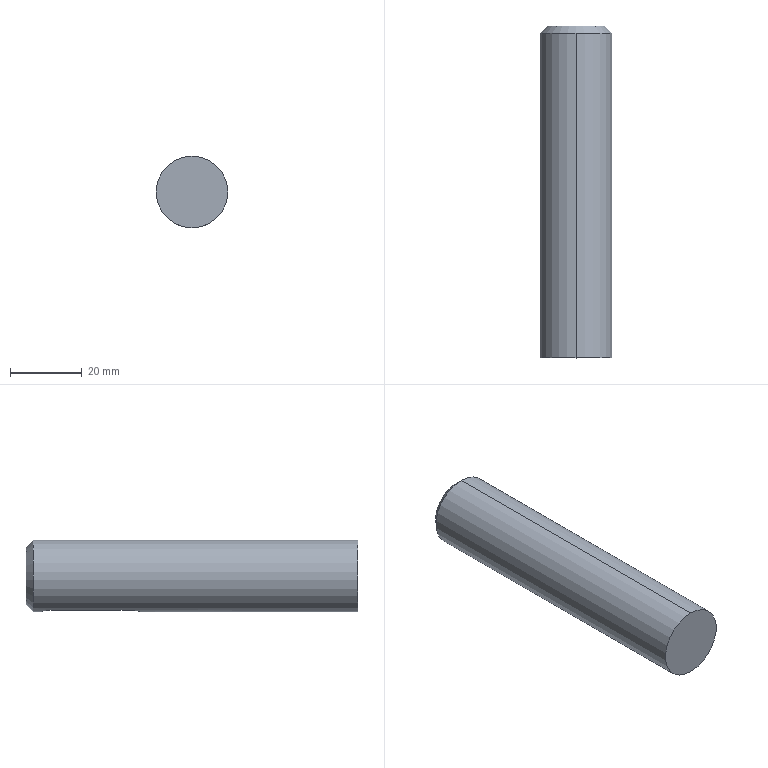Part | SolidWorks | features Chamfer 1, Extrusion 1, ICE 1 | 1 solid | 11 faces | box 20 x 92.5 x 20 mm | volume 28405 mm3 | plane 5 | cylinder 4 | cone 2 | commonest cylinder face diameters 6 x2 20 x2
STEP:
#1=CARTESIAN_POINT('',(0.,92.5,8.));
#2=VERTEX_POINT('',#1);
#3=CARTESIAN_POINT('',(0.,92.5,-8.));
#4=VERTEX_POINT('',#3);
#5=CARTESIAN_POINT('',(0.,92.5,0.));
#6=DIRECTION('',(0.,1.,0.));
#7=DIRECTION('',(0.,0.,1.));
#8=AXIS2_PLACEMENT_3D('',#5,#6,#7);
#9=CIRCLE('',#8,8.);
#10=EDGE_CURVE('',#2,#4,#9,.T.);
#11=ORIENTED_EDGE('',*,*,#10,.F.);
#12=CARTESIAN_POINT('',(0.,90.5,10.));
#13=VERTEX_POINT('',#12);
#14=CARTESIAN_POINT('',(0.,92.5,8.));
#15=DIRECTION('',(0.,-0.7071,0.7071));
#16=VECTOR('',#15,1000.);
#17=LINE('',#14,#16);
#18=EDGE_CURVE('',#2,#13,#17,.T.);
#19=ORIENTED_EDGE('',*,*,#18,.T.);
#20=CARTESIAN_POINT('',(0.,90.5,-10.));
#21=VERTEX_POINT('',#20);
#22=CARTESIAN_POINT('',(0.,90.5,0.));
#23=DIRECTION('',(0.,-1.,0.));
#24=DIRECTION('',(0.,0.,1.));
#25=AXIS2_PLACEMENT_3D('',#22,#23,#24);
#26=CIRCLE('',#25,10.);
#27=EDGE_CURVE('',#21,#13,#26,.T.);
#28=ORIENTED_EDGE('',*,*,#27,.F.);
#29=CARTESIAN_POINT('',(0.,92.5,-8.));
#30=DIRECTION('',(0.,-0.7071,-0.7071));
#31=VECTOR('',#30,1000.);
#32=LINE('',#29,#31);
#33=EDGE_CURVE('',#4,#21,#32,.T.);
#34=ORIENTED_EDGE('',*,*,#33,.F.);
#35=EDGE_LOOP('',(#11,#19,#28,#34));
#36=FACE_OUTER_BOUND('',#35,.T.);
#37=CARTESIAN_POINT('',(0.,92.5,0.));
#38=DIRECTION('',(0.,-1.,0.));
#39=DIRECTION('',(0.,0.,-1.));
#40=AXIS2_PLACEMENT_3D('',#37,#38,#39);
#41=CONICAL_SURFACE('',#40,8.,0.7854);
#42=ADVANCED_FACE('',(#36),#41,.T.);
#43=ORIENTED_EDGE('',*,*,#27,.T.);
#44=CARTESIAN_POINT('',(0.,0.,10.));
#45=VERTEX_POINT('',#44);
#46=CARTESIAN_POINT('',(0.,92.5,10.));
#47=DIRECTION('',(0.,-1.,0.));
#48=VECTOR('',#47,1000.);
#49=LINE('',#46,#48);
#50=EDGE_CURVE('',#13,#45,#49,.T.);
#51=ORIENTED_EDGE('',*,*,#50,.T.);
#52=CARTESIAN_POINT('',(0.,0.,-10.));
#53=VERTEX_POINT('',#52);
#54=CARTESIAN_POINT('',(0.,0.,0.));
#55=DIRECTION('',(0.,1.,0.));
#56=DIRECTION('',(0.,0.,1.));
#57=AXIS2_PLACEMENT_3D('',#54,#55,#56);
#58=CIRCLE('',#57,10.);
#59=EDGE_CURVE('',#45,#53,#58,.T.);
#60=ORIENTED_EDGE('',*,*,#59,.T.);
#61=CARTESIAN_POINT('',(0.,60.5,-10.));
#62=VERTEX_POINT('',#61);
#63=CARTESIAN_POINT('',(0.,92.5,-10.));
#64=DIRECTION('',(0.,-1.,0.));
#65=VECTOR('',#64,1000.);
#66=LINE('',#63,#65);
#67=EDGE_CURVE('',#62,#53,#66,.T.);
#68=ORIENTED_EDGE('',*,*,#67,.F.);
#69=CARTESIAN_POINT('',(3.,63.5,-9.539));
#70=VERTEX_POINT('',#69);
#71=CARTESIAN_POINT('',(0.,60.5,-10.));
#72=CARTESIAN_POINT('',(0.1968,60.5,-10.));
#73=CARTESIAN_POINT('',(0.3967,60.52,-9.994));
#74=CARTESIAN_POINT('',(0.7821,60.597,-9.971));
#75=CARTESIAN_POINT('',(0.9695,60.654,-9.955));
#76=CARTESIAN_POINT('',(1.334,60.806,-9.912));
#77=CARTESIAN_POINT('',(1.507,60.899,-9.887));
#78=CARTESIAN_POINT('',(1.831,61.116,-9.832));
#79=CARTESIAN_POINT('',(1.983,61.241,-9.802));
#80=CARTESIAN_POINT('',(2.26,61.517,-9.742));
#81=CARTESIAN_POINT('',(2.383,61.667,-9.713));
#82=CARTESIAN_POINT('',(2.6,61.991,-9.657));
#83=CARTESIAN_POINT('',(2.694,62.167,-9.63));
#84=CARTESIAN_POINT('',(2.845,62.528,-9.587));
#85=CARTESIAN_POINT('',(2.902,62.715,-9.57));
#86=CARTESIAN_POINT('',(2.98,63.101,-9.546));
#87=CARTESIAN_POINT('',(3.,63.301,-9.539));
#88=CARTESIAN_POINT('',(3.,63.5,-9.539));
#89=B_SPLINE_CURVE_WITH_KNOTS('',3,(#71,#72,#73,#74,#75,#76,#77,#78,#79,#80,#81,#82,#83,#84,#85,#86,#87,#88),.UNSPECIFIED.,.F.,.F.,(4,2,2,2,2,2,2,2,4),(0.004718,0.005307,0.005896,0.006485,0.007074,0.007663,0.008252,0.008842,0.009431),.UNSPECIFIED.);
#90=EDGE_CURVE('',#62,#70,#89,.T.);
#91=ORIENTED_EDGE('',*,*,#90,.T.);
#92=CARTESIAN_POINT('',(3.,85.5,-9.539));
#93=VERTEX_POINT('',#92);
#94=CARTESIAN_POINT('',(3.,92.5,-9.539));
#95=DIRECTION('',(0.,1.,0.));
#96=VECTOR('',#95,1000.);
#97=LINE('',#94,#96);
#98=EDGE_CURVE('',#70,#93,#97,.T.);
#99=ORIENTED_EDGE('',*,*,#98,.T.);
#100=CARTESIAN_POINT('',(0.,88.5,-10.));
#101=VERTEX_POINT('',#100);
#102=CARTESIAN_POINT('',(3.,85.5,-9.539));
#103=CARTESIAN_POINT('',(3.,85.7,-9.539));
#104=CARTESIAN_POINT('',(2.98,85.895,-9.546));
#105=CARTESIAN_POINT('',(2.903,86.281,-9.569));
#106=CARTESIAN_POINT('',(2.845,86.472,-9.587));
#107=CARTESIAN_POINT('',(2.694,86.835,-9.631));
#108=CARTESIAN_POINT('',(2.602,87.006,-9.656));
#109=CARTESIAN_POINT('',(2.384,87.332,-9.712));
#110=CARTESIAN_POINT('',(2.258,87.485,-9.743));
#111=CARTESIAN_POINT('',(1.845,87.897,-9.832));
#112=CARTESIAN_POINT('',(1.512,88.12,-9.892));
#113=CARTESIAN_POINT('',(0.971,88.345,-9.954));
#114=CARTESIAN_POINT('',(0.7806,88.403,-9.971));
#115=CARTESIAN_POINT('',(0.3926,88.481,-9.994));
#116=CARTESIAN_POINT('',(0.197,88.5,-10.));
#117=CARTESIAN_POINT('',(0.,88.5,-10.));
#118=B_SPLINE_CURVE_WITH_KNOTS('',3,(#102,#103,#104,#105,#106,#107,#108,#109,#110,#111,#112,#113,#114,#115,#116,#117),.UNSPECIFIED.,.F.,.F.,(4,2,2,2,2,2,2,4),(0.,0.0005898,0.00118,0.001769,0.002359,0.003539,0.004128,0.004718),.UNSPECIFIED.);
#119=EDGE_CURVE('',#93,#101,#118,.T.);
#120=ORIENTED_EDGE('',*,*,#119,.T.);
#121=CARTESIAN_POINT('',(0.,92.5,-10.));
#122=DIRECTION('',(0.,-1.,0.));
#123=VECTOR('',#122,1000.);
#124=LINE('',#121,#123);
#125=EDGE_CURVE('',#21,#101,#124,.T.);
#126=ORIENTED_EDGE('',*,*,#125,.F.);
#127=EDGE_LOOP('',(#43,#51,#60,#68,#91,#99,#120,#126));
#128=FACE_OUTER_BOUND('',#127,.T.);
#129=CARTESIAN_POINT('',(0.,92.5,0.));
#130=DIRECTION('',(0.,-1.,0.));
#131=DIRECTION('',(0.,0.,-1.));
#132=AXIS2_PLACEMENT_3D('',#129,#130,#131);
#133=CYLINDRICAL_SURFACE('',#132,10.);
#134=ADVANCED_FACE('',(#128),#133,.T.);
#135=ORIENTED_EDGE('',*,*,#50,.F.);
#136=CARTESIAN_POINT('',(0.,90.5,0.));
#137=DIRECTION('',(0.,-1.,0.));
#138=DIRECTION('',(0.,0.,1.));
#139=AXIS2_PLACEMENT_3D('',#136,#137,#138);
#140=CIRCLE('',#139,10.);
#141=EDGE_CURVE('',#13,#21,#140,.T.);
#142=ORIENTED_EDGE('',*,*,#141,.T.);
#143=ORIENTED_EDGE('',*,*,#125,.T.);
#144=CARTESIAN_POINT('',(-3.,85.5,-9.539));
#145=VERTEX_POINT('',#144);
#146=CARTESIAN_POINT('',(0.,88.5,-10.));
#147=CARTESIAN_POINT('',(-0.1968,88.5,-10.));
#148=CARTESIAN_POINT('',(-0.3967,88.48,-9.994));
#149=CARTESIAN_POINT('',(-0.7821,88.403,-9.971));
#150=CARTESIAN_POINT('',(-0.9695,88.346,-9.955));
#151=CARTESIAN_POINT('',(-1.334,88.194,-9.912));
#152=CARTESIAN_POINT('',(-1.507,88.101,-9.887));
#153=CARTESIAN_POINT('',(-1.831,87.884,-9.832));
#154=CARTESIAN_POINT('',(-1.983,87.759,-9.802));
#155=CARTESIAN_POINT('',(-2.26,87.483,-9.742));
#156=CARTESIAN_POINT('',(-2.383,87.333,-9.713));
#157=CARTESIAN_POINT('',(-2.6,87.009,-9.657));
#158=CARTESIAN_POINT('',(-2.694,86.833,-9.63));
#159=CARTESIAN_POINT('',(-2.845,86.472,-9.587));
#160=CARTESIAN_POINT('',(-2.902,86.285,-9.57));
#161=CARTESIAN_POINT('',(-2.98,85.899,-9.546));
#162=CARTESIAN_POINT('',(-3.,85.699,-9.539));
#163=CARTESIAN_POINT('',(-3.,85.5,-9.539));
#164=B_SPLINE_CURVE_WITH_KNOTS('',3,(#146,#147,#148,#149,#150,#151,#152,#153,#154,#155,#156,#157,#158,#159,#160,#161,#162,#163),.UNSPECIFIED.,.F.,.F.,(4,2,2,2,2,2,2,2,4),(0.004718,0.005307,0.005896,0.006485,0.007074,0.007663,0.008252,0.008842,0.009431),.UNSPECIFIED.);
#165=EDGE_CURVE('',#101,#145,#164,.T.);
#166=ORIENTED_EDGE('',*,*,#165,.T.);
#167=CARTESIAN_POINT('',(-3.,63.5,-9.539));
#168=VERTEX_POINT('',#167);
#169=CARTESIAN_POINT('',(-3.,92.5,-9.539));
#170=DIRECTION('',(0.,-1.,0.));
#171=VECTOR('',#170,1000.);
#172=LINE('',#169,#171);
#173=EDGE_CURVE('',#145,#168,#172,.T.);
#174=ORIENTED_EDGE('',*,*,#173,.T.);
#175=CARTESIAN_POINT('',(-3.,63.5,-9.539));
#176=CARTESIAN_POINT('',(-3.,63.3,-9.539));
#177=CARTESIAN_POINT('',(-2.98,63.105,-9.546));
#178=CARTESIAN_POINT('',(-2.903,62.719,-9.569));
#179=CARTESIAN_POINT('',(-2.845,62.528,-9.587));
#180=CARTESIAN_POINT('',(-2.694,62.165,-9.631));
#181=CARTESIAN_POINT('',(-2.602,61.994,-9.656));
#182=CARTESIAN_POINT('',(-2.384,61.668,-9.712));
#183=CARTESIAN_POINT('',(-2.258,61.515,-9.743));
#184=CARTESIAN_POINT('',(-1.845,61.103,-9.832));
#185=CARTESIAN_POINT('',(-1.512,60.88,-9.892));
#186=CARTESIAN_POINT('',(-0.971,60.655,-9.954));
#187=CARTESIAN_POINT('',(-0.7806,60.597,-9.971));
#188=CARTESIAN_POINT('',(-0.3926,60.519,-9.994));
#189=CARTESIAN_POINT('',(-0.197,60.5,-10.));
#190=CARTESIAN_POINT('',(0.,60.5,-10.));
#191=B_SPLINE_CURVE_WITH_KNOTS('',3,(#175,#176,#177,#178,#179,#180,#181,#182,#183,#184,#185,#186,#187,#188,#189,#190),.UNSPECIFIED.,.F.,.F.,(4,2,2,2,2,2,2,4),(0.,0.0005898,0.00118,0.001769,0.002359,0.003539,0.004128,0.004718),.UNSPECIFIED.);
#192=EDGE_CURVE('',#168,#62,#191,.T.);
#193=ORIENTED_EDGE('',*,*,#192,.T.);
#194=ORIENTED_EDGE('',*,*,#67,.T.);
#195=CARTESIAN_POINT('',(0.,0.,0.));
#196=DIRECTION('',(0.,1.,0.));
#197=DIRECTION('',(0.,0.,1.));
#198=AXIS2_PLACEMENT_3D('',#195,#196,#197);
#199=CIRCLE('',#198,10.);
#200=EDGE_CURVE('',#53,#45,#199,.T.);
#201=ORIENTED_EDGE('',*,*,#200,.T.);
#202=EDGE_LOOP('',(#135,#142,#143,#166,#174,#193,#194,#201));
#203=FACE_OUTER_BOUND('',#202,.T.);
#204=CARTESIAN_POINT('',(0.,92.5,0.));
#205=DIRECTION('',(0.,-1.,0.));
#206=DIRECTION('',(0.,0.,-1.));
#207=AXIS2_PLACEMENT_3D('',#204,#205,#206);
#208=CYLINDRICAL_SURFACE('',#207,10.);
#209=ADVANCED_FACE('',(#203),#208,.T.);
#210=CARTESIAN_POINT('',(0.,92.5,0.));
#211=DIRECTION('',(0.,1.,0.));
#212=DIRECTION('',(0.,0.,1.));
#213=AXIS2_PLACEMENT_3D('',#210,#211,#212);
#214=CIRCLE('',#213,8.);
#215=EDGE_CURVE('',#4,#2,#214,.T.);
#216=ORIENTED_EDGE('',*,*,#215,.T.);
#217=ORIENTED_EDGE('',*,*,#10,.T.);
#218=EDGE_LOOP('',(#216,#217));
#219=FACE_OUTER_BOUND('',#218,.T.);
#220=CARTESIAN_POINT('',(0.,92.5,0.));
#221=DIRECTION('',(0.,1.,0.));
#222=DIRECTION('',(0.,0.,1.));
#223=AXIS2_PLACEMENT_3D('',#220,#221,#222);
#224=PLANE('',#223);
#225=ADVANCED_FACE('',(#219),#224,.T.);
#226=ORIENTED_EDGE('',*,*,#200,.F.);
#227=ORIENTED_EDGE('',*,*,#59,.F.);
#228=EDGE_LOOP('',(#226,#227));
#229=FACE_OUTER_BOUND('',#228,.T.);
#230=CARTESIAN_POINT('',(0.,0.,0.));
#231=DIRECTION('',(0.,1.,0.));
#232=DIRECTION('',(0.,0.,1.));
#233=AXIS2_PLACEMENT_3D('',#230,#231,#232);
#234=PLANE('',#233);
#235=ADVANCED_FACE('',(#229),#234,.F.);
#236=CARTESIAN_POINT('',(-3.,63.5,-6.5));
#237=VERTEX_POINT('',#236);
#238=CARTESIAN_POINT('',(-3.,63.5,-10.));
#239=DIRECTION('',(0.,0.,1.));
#240=VECTOR('',#239,1000.);
#241=LINE('',#238,#240);
#242=EDGE_CURVE('',#168,#237,#241,.T.);
#243=ORIENTED_EDGE('',*,*,#242,.T.);
#244=CARTESIAN_POINT('',(3.,63.5,-6.5));
#245=VERTEX_POINT('',#244);
#246=CARTESIAN_POINT('',(0.,63.5,-6.5));
#247=DIRECTION('',(0.,0.,1.));
#248=DIRECTION('',(1.,0.,0.));
#249=AXIS2_PLACEMENT_3D('',#246,#247,#248);
#250=CIRCLE('',#249,3.);
#251=EDGE_CURVE('',#237,#245,#250,.T.);
#252=ORIENTED_EDGE('',*,*,#251,.T.);
#253=CARTESIAN_POINT('',(3.,63.5,-10.));
#254=DIRECTION('',(0.,0.,1.));
#255=VECTOR('',#254,1000.);
#256=LINE('',#253,#255);
#257=EDGE_CURVE('',#70,#245,#256,.T.);
#258=ORIENTED_EDGE('',*,*,#257,.F.);
#259=ORIENTED_EDGE('',*,*,#90,.F.);
#260=ORIENTED_EDGE('',*,*,#192,.F.);
#261=EDGE_LOOP('',(#243,#252,#258,#259,#260));
#262=FACE_OUTER_BOUND('',#261,.T.);
#263=CARTESIAN_POINT('',(0.,63.5,-10.));
#264=DIRECTION('',(0.,0.,1.));
#265=DIRECTION('',(1.,0.,0.));
#266=AXIS2_PLACEMENT_3D('',#263,#264,#265);
#267=CYLINDRICAL_SURFACE('',#266,3.);
#268=ADVANCED_FACE('',(#262),#267,.F.);
#269=CARTESIAN_POINT('',(-3.,85.5,-6.5));
#270=VERTEX_POINT('',#269);
#271=CARTESIAN_POINT('',(-3.,85.5,-10.));
#272=DIRECTION('',(0.,0.,1.));
#273=VECTOR('',#272,1000.);
#274=LINE('',#271,#273);
#275=EDGE_CURVE('',#145,#270,#274,.T.);
#276=ORIENTED_EDGE('',*,*,#275,.T.);
#277=CARTESIAN_POINT('',(-3.,63.5,-6.5));
#278=DIRECTION('',(0.,-1.,0.));
#279=VECTOR('',#278,1000.);
#280=LINE('',#277,#279);
#281=EDGE_CURVE('',#270,#237,#280,.T.);
#282=ORIENTED_EDGE('',*,*,#281,.T.);
#283=ORIENTED_EDGE('',*,*,#242,.F.);
#284=ORIENTED_EDGE('',*,*,#173,.F.);
#285=EDGE_LOOP('',(#276,#282,#283,#284));
#286=FACE_OUTER_BOUND('',#285,.T.);
#287=CARTESIAN_POINT('',(-3.,63.5,-10.));
#288=DIRECTION('',(-1.,0.,0.));
#289=DIRECTION('',(0.,-1.,0.));
#290=AXIS2_PLACEMENT_3D('',#287,#288,#289);
#291=PLANE('',#290);
#292=ADVANCED_FACE('',(#286),#291,.F.);
#293=CARTESIAN_POINT('',(3.,85.5,-6.5));
#294=VERTEX_POINT('',#293);
#295=CARTESIAN_POINT('',(3.,85.5,-10.));
#296=DIRECTION('',(0.,0.,1.));
#297=VECTOR('',#296,1000.);
#298=LINE('',#295,#297);
#299=EDGE_CURVE('',#93,#294,#298,.T.);
#300=ORIENTED_EDGE('',*,*,#299,.T.);
#301=CARTESIAN_POINT('',(0.,85.5,-6.5));
#302=DIRECTION('',(0.,0.,1.));
#303=DIRECTION('',(1.,0.,0.));
#304=AXIS2_PLACEMENT_3D('',#301,#302,#303);
#305=CIRCLE('',#304,3.);
#306=EDGE_CURVE('',#294,#270,#305,.T.);
#307=ORIENTED_EDGE('',*,*,#306,.T.);
#308=ORIENTED_EDGE('',*,*,#275,.F.);
#309=ORIENTED_EDGE('',*,*,#165,.F.);
#310=ORIENTED_EDGE('',*,*,#119,.F.);
#311=EDGE_LOOP('',(#300,#307,#308,#309,#310));
#312=FACE_OUTER_BOUND('',#311,.T.);
#313=CARTESIAN_POINT('',(0.,85.5,-10.));
#314=DIRECTION('',(0.,0.,1.));
#315=DIRECTION('',(1.,0.,0.));
#316=AXIS2_PLACEMENT_3D('',#313,#314,#315);
#317=CYLINDRICAL_SURFACE('',#316,3.);
#318=ADVANCED_FACE('',(#312),#317,.F.);
#319=ORIENTED_EDGE('',*,*,#257,.T.);
#320=CARTESIAN_POINT('',(3.,63.5,-6.5));
#321=DIRECTION('',(0.,1.,0.));
#322=VECTOR('',#321,1000.);
#323=LINE('',#320,#322);
#324=EDGE_CURVE('',#245,#294,#323,.T.);
#325=ORIENTED_EDGE('',*,*,#324,.T.);
#326=ORIENTED_EDGE('',*,*,#299,.F.);
#327=ORIENTED_EDGE('',*,*,#98,.F.);
#328=EDGE_LOOP('',(#319,#325,#326,#327));
#329=FACE_OUTER_BOUND('',#328,.T.);
#330=CARTESIAN_POINT('',(3.,63.5,-10.));
#331=DIRECTION('',(1.,0.,0.));
#332=DIRECTION('',(0.,1.,0.));
#333=AXIS2_PLACEMENT_3D('',#330,#331,#332);
#334=PLANE('',#333);
#335=ADVANCED_FACE('',(#329),#334,.F.);
#336=ORIENTED_EDGE('',*,*,#251,.F.);
#337=ORIENTED_EDGE('',*,*,#281,.F.);
#338=ORIENTED_EDGE('',*,*,#306,.F.);
#339=ORIENTED_EDGE('',*,*,#324,.F.);
#340=EDGE_LOOP('',(#336,#337,#338,#339));
#341=FACE_OUTER_BOUND('',#340,.T.);
#342=CARTESIAN_POINT('',(0.,63.5,-6.5));
#343=DIRECTION('',(0.,0.,1.));
#344=DIRECTION('',(1.,0.,0.));
#345=AXIS2_PLACEMENT_3D('',#342,#343,#344);
#346=PLANE('',#345);
#347=ADVANCED_FACE('',(#341),#346,.F.);
#348=ORIENTED_EDGE('',*,*,#18,.F.);
#349=ORIENTED_EDGE('',*,*,#215,.F.);
#350=ORIENTED_EDGE('',*,*,#33,.T.);
#351=ORIENTED_EDGE('',*,*,#141,.F.);
#352=EDGE_LOOP('',(#348,#349,#350,#351));
#353=FACE_OUTER_BOUND('',#352,.T.);
#354=CARTESIAN_POINT('',(0.,92.5,0.));
#355=DIRECTION('',(0.,-1.,0.));
#356=DIRECTION('',(0.,0.,-1.));
#357=AXIS2_PLACEMENT_3D('',#354,#355,#356);
#358=CONICAL_SURFACE('',#357,8.,0.7854);
#359=ADVANCED_FACE('',(#353),#358,.T.);
#360=CLOSED_SHELL('',(#42,#134,#209,#225,#235,#268,#292,#318,#335,#347,#359));
#361=MANIFOLD_SOLID_BREP('',#360);
#362=CARTESIAN_POINT('',(0.,0.,0.));
#363=DIRECTION('',(0.,0.,1.));
#364=DIRECTION('',(1.,0.,0.));
#365=AXIS2_PLACEMENT_3D('',#362,#363,#364);
#366=(LENGTH_UNIT()NAMED_UNIT(*)SI_UNIT(.MILLI.,.METRE.));
#367=UNCERTAINTY_MEASURE_WITH_UNIT(LENGTH_MEASURE(0.00001),#366,'','');
#368=(NAMED_UNIT(*)PLANE_ANGLE_UNIT()SI_UNIT($,.RADIAN.));
#369=(NAMED_UNIT(*)SI_UNIT($,.STERADIAN.)SOLID_ANGLE_UNIT());
#370=(GEOMETRIC_REPRESENTATION_CONTEXT(3)GLOBAL_UNCERTAINTY_ASSIGNED_CONTEXT((#367))GLOBAL_UNIT_ASSIGNED_CONTEXT((#366,#368,#369))REPRESENTATION_CONTEXT('',''));
#371=ADVANCED_BREP_SHAPE_REPRESENTATION('',(#361,#365),#370);